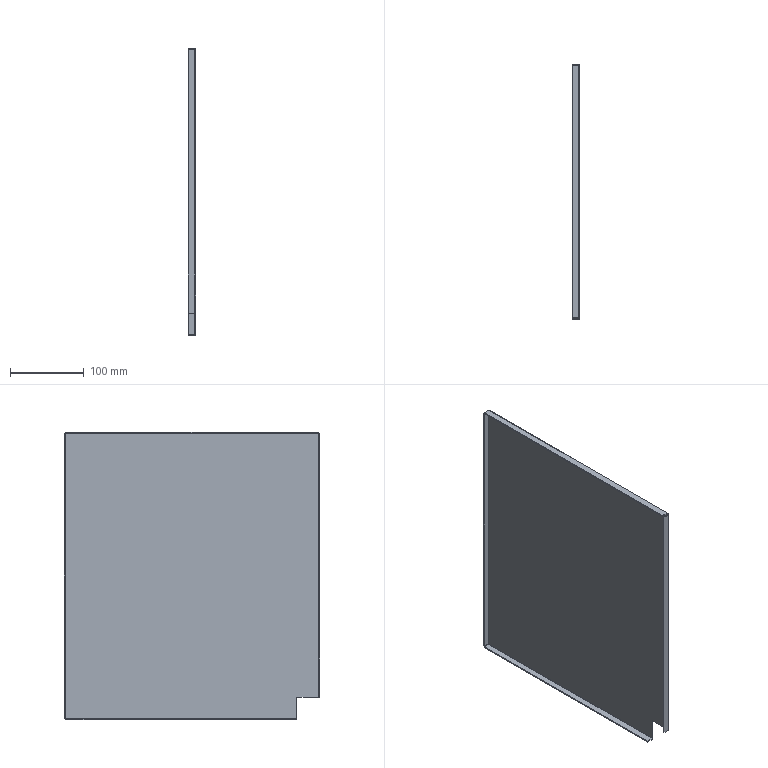Part | SolidWorks | 1 solid | 36 faces | box 10 x 346.001 x 390.001 mm | volume 217996 mm3 | plane 22 | cylinder 8 | spline 6 | commonest cylinder face diameters 0.2 x4 3.2 x4
STEP:
#1=CARTESIAN_POINT('',(-1.5,-142.,-193.4));
#2=VERTEX_POINT('',#1);
#3=CARTESIAN_POINT('',(-1.5,-142.,-164.));
#4=VERTEX_POINT('',#3);
#5=CARTESIAN_POINT('',(-1.5,-142.,0.));
#6=DIRECTION('',(0.,0.,1.));
#7=VECTOR('',#6,1000.);
#8=LINE('',#5,#7);
#9=EDGE_CURVE('',#2,#4,#8,.T.);
#10=ORIENTED_EDGE('',*,*,#9,.T.);
#11=CARTESIAN_POINT('',(-1.5,-171.4,-164.));
#12=VERTEX_POINT('',#11);
#13=CARTESIAN_POINT('',(-1.5,0.,-164.));
#14=DIRECTION('',(0.,-1.,0.));
#15=VECTOR('',#14,1000.);
#16=LINE('',#13,#15);
#17=EDGE_CURVE('',#4,#12,#16,.T.);
#18=ORIENTED_EDGE('',*,*,#17,.T.);
#19=CARTESIAN_POINT('',(-1.5,-171.4,193.4));
#20=VERTEX_POINT('',#19);
#21=CARTESIAN_POINT('',(-1.5,-171.4,193.4));
#22=DIRECTION('',(0.,0.,-1.));
#23=VECTOR('',#22,1000.);
#24=LINE('',#21,#23);
#25=EDGE_CURVE('',#20,#12,#24,.T.);
#26=ORIENTED_EDGE('',*,*,#25,.F.);
#27=CARTESIAN_POINT('',(-1.5,171.4,193.4));
#28=VERTEX_POINT('',#27);
#29=CARTESIAN_POINT('',(-1.5,171.4,193.4));
#30=DIRECTION('',(0.,-1.,0.));
#31=VECTOR('',#30,1000.);
#32=LINE('',#29,#31);
#33=EDGE_CURVE('',#28,#20,#32,.T.);
#34=ORIENTED_EDGE('',*,*,#33,.F.);
#35=CARTESIAN_POINT('',(-1.5,171.4,-193.4));
#36=VERTEX_POINT('',#35);
#37=CARTESIAN_POINT('',(-1.5,171.4,-193.4));
#38=DIRECTION('',(0.,0.,1.));
#39=VECTOR('',#38,1000.);
#40=LINE('',#37,#39);
#41=EDGE_CURVE('',#36,#28,#40,.T.);
#42=ORIENTED_EDGE('',*,*,#41,.F.);
#43=CARTESIAN_POINT('',(-1.5,-171.4,-193.4));
#44=DIRECTION('',(0.,1.,0.));
#45=VECTOR('',#44,1000.);
#46=LINE('',#43,#45);
#47=EDGE_CURVE('',#2,#36,#46,.T.);
#48=ORIENTED_EDGE('',*,*,#47,.F.);
#49=EDGE_LOOP('',(#10,#18,#26,#34,#42,#48));
#50=FACE_OUTER_BOUND('',#49,.T.);
#51=CARTESIAN_POINT('',(-1.5,0.,0.));
#52=DIRECTION('',(1.,0.,0.));
#53=DIRECTION('',(0.,0.,-1.));
#54=AXIS2_PLACEMENT_3D('',#51,#52,#53);
#55=PLANE('',#54);
#56=ADVANCED_FACE('',(#50),#55,.F.);
#57=CARTESIAN_POINT('',(0.,-142.,-164.));
#58=VERTEX_POINT('',#57);
#59=CARTESIAN_POINT('',(0.,-171.4,-164.));
#60=VERTEX_POINT('',#59);
#61=CARTESIAN_POINT('',(0.,-182.,-164.));
#62=DIRECTION('',(0.,-1.,0.));
#63=VECTOR('',#62,1000.);
#64=LINE('',#61,#63);
#65=EDGE_CURVE('',#58,#60,#64,.T.);
#66=ORIENTED_EDGE('',*,*,#65,.F.);
#67=CARTESIAN_POINT('',(0.,-142.,-193.4));
#68=VERTEX_POINT('',#67);
#69=CARTESIAN_POINT('',(0.,-142.,-204.));
#70=DIRECTION('',(0.,0.,1.));
#71=VECTOR('',#70,1000.);
#72=LINE('',#69,#71);
#73=EDGE_CURVE('',#68,#58,#72,.T.);
#74=ORIENTED_EDGE('',*,*,#73,.F.);
#75=CARTESIAN_POINT('',(0.,171.4,-193.4));
#76=VERTEX_POINT('',#75);
#77=CARTESIAN_POINT('',(0.,-171.4,-193.4));
#78=DIRECTION('',(0.,1.,0.));
#79=VECTOR('',#78,1000.);
#80=LINE('',#77,#79);
#81=EDGE_CURVE('',#68,#76,#80,.T.);
#82=ORIENTED_EDGE('',*,*,#81,.T.);
#83=CARTESIAN_POINT('',(0.,171.4,193.4));
#84=VERTEX_POINT('',#83);
#85=CARTESIAN_POINT('',(0.,171.4,-193.4));
#86=DIRECTION('',(0.,0.,1.));
#87=VECTOR('',#86,1000.);
#88=LINE('',#85,#87);
#89=EDGE_CURVE('',#76,#84,#88,.T.);
#90=ORIENTED_EDGE('',*,*,#89,.T.);
#91=CARTESIAN_POINT('',(0.,-171.4,193.4));
#92=VERTEX_POINT('',#91);
#93=CARTESIAN_POINT('',(0.,171.4,193.4));
#94=DIRECTION('',(0.,-1.,0.));
#95=VECTOR('',#94,1000.);
#96=LINE('',#93,#95);
#97=EDGE_CURVE('',#84,#92,#96,.T.);
#98=ORIENTED_EDGE('',*,*,#97,.T.);
#99=CARTESIAN_POINT('',(0.,-171.4,193.4));
#100=DIRECTION('',(0.,0.,-1.));
#101=VECTOR('',#100,1000.);
#102=LINE('',#99,#101);
#103=EDGE_CURVE('',#92,#60,#102,.T.);
#104=ORIENTED_EDGE('',*,*,#103,.T.);
#105=EDGE_LOOP('',(#66,#74,#82,#90,#98,#104));
#106=FACE_OUTER_BOUND('',#105,.T.);
#107=CARTESIAN_POINT('',(0.,0.,0.));
#108=DIRECTION('',(1.,0.,0.));
#109=DIRECTION('',(0.,0.,-1.));
#110=AXIS2_PLACEMENT_3D('',#107,#108,#109);
#111=PLANE('',#110);
#112=ADVANCED_FACE('',(#106),#111,.T.);
#113=CARTESIAN_POINT('',(-1.6,173.,192.793));
#114=VERTEX_POINT('',#113);
#115=CARTESIAN_POINT('',(-1.6,171.5,192.793));
#116=VERTEX_POINT('',#115);
#117=CARTESIAN_POINT('',(-1.6,171.5,192.793));
#118=DIRECTION('',(0.,-1.,0.));
#119=VECTOR('',#118,1000.);
#120=LINE('',#117,#119);
#121=EDGE_CURVE('',#114,#116,#120,.T.);
#122=ORIENTED_EDGE('',*,*,#121,.T.);
#123=CARTESIAN_POINT('',(-1.5,171.4,193.4));
#124=CARTESIAN_POINT('',(-1.5,171.426,193.299));
#125=CARTESIAN_POINT('',(-1.511,171.452,193.198));
#126=CARTESIAN_POINT('',(-1.548,171.489,192.995));
#127=CARTESIAN_POINT('',(-1.574,171.5,192.894));
#128=CARTESIAN_POINT('',(-1.6,171.5,192.793));
#129=B_SPLINE_CURVE_WITH_KNOTS('',3,(#123,#124,#125,#126,#127,#128),.UNSPECIFIED.,.F.,.F.,(4,2,4),(0.,0.5,1.),.UNSPECIFIED.);
#130=EDGE_CURVE('',#28,#116,#129,.T.);
#131=ORIENTED_EDGE('',*,*,#130,.F.);
#132=CARTESIAN_POINT('',(-1.5,171.4,193.4));
#133=DIRECTION('',(1.,0.,0.));
#134=VECTOR('',#133,1000.);
#135=LINE('',#132,#134);
#136=EDGE_CURVE('',#28,#84,#135,.T.);
#137=ORIENTED_EDGE('',*,*,#136,.T.);
#138=CARTESIAN_POINT('',(0.,171.4,193.4));
#139=CARTESIAN_POINT('',(0.,171.612,193.349));
#140=CARTESIAN_POINT('',(-0.04048,171.815,193.3));
#141=CARTESIAN_POINT('',(-0.2012,172.205,193.198));
#142=CARTESIAN_POINT('',(-0.3186,172.381,193.148));
#143=CARTESIAN_POINT('',(-0.5418,172.605,193.071));
#144=CARTESIAN_POINT('',(-0.6225,172.671,193.046));
#145=CARTESIAN_POINT('',(-0.7959,172.787,192.996));
#146=CARTESIAN_POINT('',(-0.8897,172.838,192.97));
#147=CARTESIAN_POINT('',(-1.18,172.958,192.894));
#148=CARTESIAN_POINT('',(-1.388,173.,192.844));
#149=CARTESIAN_POINT('',(-1.6,173.,192.793));
#150=B_SPLINE_CURVE_WITH_KNOTS('',3,(#138,#139,#140,#141,#142,#143,#144,#145,#146,#147,#148,#149),.UNSPECIFIED.,.F.,.F.,(4,2,2,2,2,4),(0.,0.0006399,0.00128,0.0016,0.00192,0.00256),.UNSPECIFIED.);
#151=EDGE_CURVE('',#84,#114,#150,.T.);
#152=ORIENTED_EDGE('',*,*,#151,.T.);
#153=EDGE_LOOP('',(#122,#131,#137,#152));
#154=FACE_OUTER_BOUND('',#153,.T.);
#155=CARTESIAN_POINT('',(0.015,171.4,193.4));
#156=CARTESIAN_POINT('',(0.015,171.611,193.349));
#157=CARTESIAN_POINT('',(-0.02703,171.823,193.299));
#158=CARTESIAN_POINT('',(-0.1888,172.213,193.198));
#159=CARTESIAN_POINT('',(-0.3085,172.392,193.147));
#160=CARTESIAN_POINT('',(-0.6075,172.691,193.046));
#161=CARTESIAN_POINT('',(-0.7867,172.811,192.995));
#162=CARTESIAN_POINT('',(-1.177,172.973,192.894));
#163=CARTESIAN_POINT('',(-1.389,173.015,192.843));
#164=CARTESIAN_POINT('',(-1.6,173.015,192.793));
#165=CARTESIAN_POINT('',(0.,171.4,193.4));
#166=CARTESIAN_POINT('',(0.,171.609,193.349));
#167=CARTESIAN_POINT('',(-0.04164,171.819,193.299));
#168=CARTESIAN_POINT('',(-0.2019,172.206,193.198));
#169=CARTESIAN_POINT('',(-0.3205,172.383,193.147));
#170=CARTESIAN_POINT('',(-0.6167,172.679,193.046));
#171=CARTESIAN_POINT('',(-0.7942,172.798,192.995));
#172=CARTESIAN_POINT('',(-1.181,172.958,192.894));
#173=CARTESIAN_POINT('',(-1.391,173.,192.843));
#174=CARTESIAN_POINT('',(-1.6,173.,192.793));
#175=CARTESIAN_POINT('',(-1.5,171.4,193.4));
#176=CARTESIAN_POINT('',(-1.5,171.413,193.349));
#177=CARTESIAN_POINT('',(-1.503,171.426,193.299));
#178=CARTESIAN_POINT('',(-1.513,171.45,193.198));
#179=CARTESIAN_POINT('',(-1.52,171.461,193.147));
#180=CARTESIAN_POINT('',(-1.539,171.48,193.046));
#181=CARTESIAN_POINT('',(-1.55,171.487,192.995));
#182=CARTESIAN_POINT('',(-1.574,171.497,192.894));
#183=CARTESIAN_POINT('',(-1.587,171.5,192.843));
#184=CARTESIAN_POINT('',(-1.6,171.5,192.793));
#185=B_SPLINE_SURFACE_WITH_KNOTS('',1,3,((#155,#156,#157,#158,#159,#160,#161,#162,#163,#164),(#165,#166,#167,#168,#169,#170,#171,#172,#173,#174),(#175,#176,#177,#178,#179,#180,#181,#182,#183,#184)),.UNSPECIFIED.,.F.,.F.,.F.,(2,1,2),(4,2,2,2,4),(-0.01,0.,1.),(0.,0.25,0.5,0.75,1.),.UNSPECIFIED.);
#186=ADVANCED_FACE('',(#154),#185,.F.);
#187=CARTESIAN_POINT('',(-1.6,171.5,-192.793));
#188=VERTEX_POINT('',#187);
#189=CARTESIAN_POINT('',(-1.6,171.5,-192.793));
#190=CARTESIAN_POINT('',(-1.574,171.5,-192.894));
#191=CARTESIAN_POINT('',(-1.548,171.489,-192.995));
#192=CARTESIAN_POINT('',(-1.511,171.452,-193.198));
#193=CARTESIAN_POINT('',(-1.5,171.426,-193.299));
#194=CARTESIAN_POINT('',(-1.5,171.4,-193.4));
#195=B_SPLINE_CURVE_WITH_KNOTS('',3,(#189,#190,#191,#192,#193,#194),.UNSPECIFIED.,.F.,.F.,(4,2,4),(0.,0.5,1.),.UNSPECIFIED.);
#196=EDGE_CURVE('',#188,#36,#195,.T.);
#197=ORIENTED_EDGE('',*,*,#196,.F.);
#198=CARTESIAN_POINT('',(-1.6,173.,-192.793));
#199=VERTEX_POINT('',#198);
#200=CARTESIAN_POINT('',(-1.6,171.5,-192.793));
#201=DIRECTION('',(0.,-1.,0.));
#202=VECTOR('',#201,1000.);
#203=LINE('',#200,#202);
#204=EDGE_CURVE('',#199,#188,#203,.T.);
#205=ORIENTED_EDGE('',*,*,#204,.F.);
#206=CARTESIAN_POINT('',(-1.6,173.,-192.793));
#207=CARTESIAN_POINT('',(-1.388,173.,-192.844));
#208=CARTESIAN_POINT('',(-1.185,172.96,-192.893));
#209=CARTESIAN_POINT('',(-0.7952,172.799,-192.995));
#210=CARTESIAN_POINT('',(-0.619,172.681,-193.045));
#211=CARTESIAN_POINT('',(-0.3953,172.458,-193.121));
#212=CARTESIAN_POINT('',(-0.329,172.378,-193.147));
#213=CARTESIAN_POINT('',(-0.2128,172.204,-193.197));
#214=CARTESIAN_POINT('',(-0.1625,172.11,-193.223));
#215=CARTESIAN_POINT('',(-0.04195,171.82,-193.299));
#216=CARTESIAN_POINT('',(0.,171.612,-193.349));
#217=CARTESIAN_POINT('',(0.,171.4,-193.4));
#218=B_SPLINE_CURVE_WITH_KNOTS('',3,(#206,#207,#208,#209,#210,#211,#212,#213,#214,#215,#216,#217),.UNSPECIFIED.,.F.,.F.,(4,2,2,2,2,4),(0.,0.0006399,0.00128,0.0016,0.00192,0.00256),.UNSPECIFIED.);
#219=EDGE_CURVE('',#199,#76,#218,.T.);
#220=ORIENTED_EDGE('',*,*,#219,.T.);
#221=CARTESIAN_POINT('',(-1.5,171.4,-193.4));
#222=DIRECTION('',(1.,0.,0.));
#223=VECTOR('',#222,1000.);
#224=LINE('',#221,#223);
#225=EDGE_CURVE('',#36,#76,#224,.T.);
#226=ORIENTED_EDGE('',*,*,#225,.F.);
#227=EDGE_LOOP('',(#197,#205,#220,#226));
#228=FACE_OUTER_BOUND('',#227,.T.);
#229=CARTESIAN_POINT('',(-1.6,173.015,-192.793));
#230=CARTESIAN_POINT('',(-1.389,173.015,-192.843));
#231=CARTESIAN_POINT('',(-1.177,172.973,-192.894));
#232=CARTESIAN_POINT('',(-0.7867,172.811,-192.995));
#233=CARTESIAN_POINT('',(-0.6075,172.691,-193.046));
#234=CARTESIAN_POINT('',(-0.3085,172.392,-193.147));
#235=CARTESIAN_POINT('',(-0.1888,172.213,-193.198));
#236=CARTESIAN_POINT('',(-0.02703,171.823,-193.299));
#237=CARTESIAN_POINT('',(0.015,171.611,-193.349));
#238=CARTESIAN_POINT('',(0.015,171.4,-193.4));
#239=CARTESIAN_POINT('',(-1.6,173.,-192.793));
#240=CARTESIAN_POINT('',(-1.391,173.,-192.843));
#241=CARTESIAN_POINT('',(-1.181,172.958,-192.894));
#242=CARTESIAN_POINT('',(-0.7942,172.798,-192.995));
#243=CARTESIAN_POINT('',(-0.6167,172.679,-193.046));
#244=CARTESIAN_POINT('',(-0.3205,172.383,-193.147));
#245=CARTESIAN_POINT('',(-0.2019,172.206,-193.198));
#246=CARTESIAN_POINT('',(-0.04164,171.819,-193.299));
#247=CARTESIAN_POINT('',(0.,171.609,-193.349));
#248=CARTESIAN_POINT('',(0.,171.4,-193.4));
#249=CARTESIAN_POINT('',(-1.6,171.5,-192.793));
#250=CARTESIAN_POINT('',(-1.587,171.5,-192.843));
#251=CARTESIAN_POINT('',(-1.574,171.497,-192.894));
#252=CARTESIAN_POINT('',(-1.55,171.487,-192.995));
#253=CARTESIAN_POINT('',(-1.539,171.48,-193.046));
#254=CARTESIAN_POINT('',(-1.52,171.461,-193.147));
#255=CARTESIAN_POINT('',(-1.513,171.45,-193.198));
#256=CARTESIAN_POINT('',(-1.503,171.426,-193.299));
#257=CARTESIAN_POINT('',(-1.5,171.413,-193.349));
#258=CARTESIAN_POINT('',(-1.5,171.4,-193.4));
#259=B_SPLINE_SURFACE_WITH_KNOTS('',1,3,((#229,#230,#231,#232,#233,#234,#235,#236,#237,#238),(#239,#240,#241,#242,#243,#244,#245,#246,#247,#248),(#249,#250,#251,#252,#253,#254,#255,#256,#257,#258)),.UNSPECIFIED.,.F.,.F.,.F.,(2,1,2),(4,2,2,2,4),(-0.01,0.,1.),(0.,0.25,0.5,0.75,1.),.UNSPECIFIED.);
#260=ADVANCED_FACE('',(#228),#259,.F.);
#261=ORIENTED_EDGE('',*,*,#89,.F.);
#262=ORIENTED_EDGE('',*,*,#219,.F.);
#263=CARTESIAN_POINT('',(-1.6,173.,0.));
#264=DIRECTION('',(0.,0.,-1.));
#265=VECTOR('',#264,1000.);
#266=LINE('',#263,#265);
#267=EDGE_CURVE('',#114,#199,#266,.T.);
#268=ORIENTED_EDGE('',*,*,#267,.F.);
#269=ORIENTED_EDGE('',*,*,#151,.F.);
#270=EDGE_LOOP('',(#261,#262,#268,#269));
#271=FACE_OUTER_BOUND('',#270,.T.);
#272=CARTESIAN_POINT('',(-1.6,171.4,-193.4));
#273=DIRECTION('',(0.,0.,-1.));
#274=DIRECTION('',(0.,1.,0.));
#275=AXIS2_PLACEMENT_3D('',#272,#273,#274);
#276=CYLINDRICAL_SURFACE('',#275,1.6);
#277=ADVANCED_FACE('',(#271),#276,.T.);
#278=ORIENTED_EDGE('',*,*,#41,.T.);
#279=ORIENTED_EDGE('',*,*,#130,.T.);
#280=CARTESIAN_POINT('',(-1.6,171.5,195.));
#281=DIRECTION('',(0.,0.,-1.));
#282=VECTOR('',#281,1000.);
#283=LINE('',#280,#282);
#284=EDGE_CURVE('',#116,#188,#283,.T.);
#285=ORIENTED_EDGE('',*,*,#284,.T.);
#286=ORIENTED_EDGE('',*,*,#196,.T.);
#287=EDGE_LOOP('',(#278,#279,#285,#286));
#288=FACE_OUTER_BOUND('',#287,.T.);
#289=CARTESIAN_POINT('',(-1.6,171.4,-193.4));
#290=DIRECTION('',(0.,0.,-1.));
#291=DIRECTION('',(0.,1.,0.));
#292=AXIS2_PLACEMENT_3D('',#289,#290,#291);
#293=CYLINDRICAL_SURFACE('',#292,0.1);
#294=ADVANCED_FACE('',(#288),#293,.F.);
#295=CARTESIAN_POINT('',(-10.,171.5,192.793));
#296=VERTEX_POINT('',#295);
#297=CARTESIAN_POINT('',(-10.,173.,192.793));
#298=VERTEX_POINT('',#297);
#299=CARTESIAN_POINT('',(-10.,173.,192.793));
#300=DIRECTION('',(0.,1.,0.));
#301=VECTOR('',#300,1000.);
#302=LINE('',#299,#301);
#303=EDGE_CURVE('',#296,#298,#302,.T.);
#304=ORIENTED_EDGE('',*,*,#303,.F.);
#305=CARTESIAN_POINT('',(0.,171.5,192.793));
#306=DIRECTION('',(-1.,0.,0.));
#307=VECTOR('',#306,1000.);
#308=LINE('',#305,#307);
#309=EDGE_CURVE('',#116,#296,#308,.T.);
#310=ORIENTED_EDGE('',*,*,#309,.F.);
#311=ORIENTED_EDGE('',*,*,#121,.F.);
#312=CARTESIAN_POINT('',(0.,173.,192.793));
#313=DIRECTION('',(1.,0.,0.));
#314=VECTOR('',#313,1000.);
#315=LINE('',#312,#314);
#316=EDGE_CURVE('',#298,#114,#315,.T.);
#317=ORIENTED_EDGE('',*,*,#316,.F.);
#318=EDGE_LOOP('',(#304,#310,#311,#317));
#319=FACE_OUTER_BOUND('',#318,.T.);
#320=CARTESIAN_POINT('',(-1.5,171.5,192.793));
#321=DIRECTION('',(0.,0.,1.));
#322=DIRECTION('',(1.,0.,0.));
#323=AXIS2_PLACEMENT_3D('',#320,#321,#322);
#324=PLANE('',#323);
#325=ADVANCED_FACE('',(#319),#324,.T.);
#326=CARTESIAN_POINT('',(-10.,173.,-192.793));
#327=VERTEX_POINT('',#326);
#328=CARTESIAN_POINT('',(-1.5,173.,-192.793));
#329=DIRECTION('',(1.,0.,0.));
#330=VECTOR('',#329,1000.);
#331=LINE('',#328,#330);
#332=EDGE_CURVE('',#327,#199,#331,.T.);
#333=ORIENTED_EDGE('',*,*,#332,.F.);
#334=CARTESIAN_POINT('',(-10.,173.,-195.));
#335=DIRECTION('',(0.,0.,-1.));
#336=VECTOR('',#335,1000.);
#337=LINE('',#334,#336);
#338=EDGE_CURVE('',#298,#327,#337,.T.);
#339=ORIENTED_EDGE('',*,*,#338,.F.);
#340=ORIENTED_EDGE('',*,*,#316,.T.);
#341=ORIENTED_EDGE('',*,*,#267,.T.);
#342=EDGE_LOOP('',(#333,#339,#340,#341));
#343=FACE_OUTER_BOUND('',#342,.T.);
#344=CARTESIAN_POINT('',(0.,173.,0.));
#345=DIRECTION('',(0.,1.,0.));
#346=DIRECTION('',(-1.,0.,0.));
#347=AXIS2_PLACEMENT_3D('',#344,#345,#346);
#348=PLANE('',#347);
#349=ADVANCED_FACE('',(#343),#348,.T.);
#350=CARTESIAN_POINT('',(-10.,171.5,-192.793));
#351=VERTEX_POINT('',#350);
#352=CARTESIAN_POINT('',(-10.,171.5,0.));
#353=DIRECTION('',(0.,0.,-1.));
#354=VECTOR('',#353,1000.);
#355=LINE('',#352,#354);
#356=EDGE_CURVE('',#296,#351,#355,.T.);
#357=ORIENTED_EDGE('',*,*,#356,.T.);
#358=CARTESIAN_POINT('',(-1.5,171.5,-192.793));
#359=DIRECTION('',(-1.,0.,0.));
#360=VECTOR('',#359,1000.);
#361=LINE('',#358,#360);
#362=EDGE_CURVE('',#188,#351,#361,.T.);
#363=ORIENTED_EDGE('',*,*,#362,.F.);
#364=ORIENTED_EDGE('',*,*,#284,.F.);
#365=ORIENTED_EDGE('',*,*,#309,.T.);
#366=EDGE_LOOP('',(#357,#363,#364,#365));
#367=FACE_OUTER_BOUND('',#366,.T.);
#368=CARTESIAN_POINT('',(0.,171.5,0.));
#369=DIRECTION('',(0.,1.,0.));
#370=DIRECTION('',(-1.,0.,0.));
#371=AXIS2_PLACEMENT_3D('',#368,#369,#370);
#372=PLANE('',#371);
#373=ADVANCED_FACE('',(#367),#372,.F.);
#374=CARTESIAN_POINT('',(-10.,171.5,-192.793));
#375=DIRECTION('',(0.,1.,0.));
#376=VECTOR('',#375,1000.);
#377=LINE('',#374,#376);
#378=EDGE_CURVE('',#351,#327,#377,.T.);
#379=ORIENTED_EDGE('',*,*,#378,.F.);
#380=ORIENTED_EDGE('',*,*,#356,.F.);
#381=ORIENTED_EDGE('',*,*,#303,.T.);
#382=ORIENTED_EDGE('',*,*,#338,.T.);
#383=EDGE_LOOP('',(#379,#380,#381,#382));
#384=FACE_OUTER_BOUND('',#383,.T.);
#385=CARTESIAN_POINT('',(-10.,173.,-195.));
#386=DIRECTION('',(-1.,0.,0.));
#387=DIRECTION('',(0.,-1.,0.));
#388=AXIS2_PLACEMENT_3D('',#385,#386,#387);
#389=PLANE('',#388);
#390=ADVANCED_FACE('',(#384),#389,.T.);
#391=ORIENTED_EDGE('',*,*,#362,.T.);
#392=ORIENTED_EDGE('',*,*,#378,.T.);
#393=ORIENTED_EDGE('',*,*,#332,.T.);
#394=ORIENTED_EDGE('',*,*,#204,.T.);
#395=EDGE_LOOP('',(#391,#392,#393,#394));
#396=FACE_OUTER_BOUND('',#395,.T.);
#397=CARTESIAN_POINT('',(-1.5,171.5,-192.793));
#398=DIRECTION('',(0.,0.,1.));
#399=DIRECTION('',(1.,0.,0.));
#400=AXIS2_PLACEMENT_3D('',#397,#398,#399);
#401=PLANE('',#400);
#402=ADVANCED_FACE('',(#396),#401,.F.);
#403=CARTESIAN_POINT('',(-1.6,-170.793,195.));
#404=VERTEX_POINT('',#403);
#405=CARTESIAN_POINT('',(-1.6,-170.793,193.5));
#406=VERTEX_POINT('',#405);
#407=CARTESIAN_POINT('',(-1.6,-170.793,193.5));
#408=DIRECTION('',(0.,0.,-1.));
#409=VECTOR('',#408,1000.);
#410=LINE('',#407,#409);
#411=EDGE_CURVE('',#404,#406,#410,.T.);
#412=ORIENTED_EDGE('',*,*,#411,.T.);
#413=CARTESIAN_POINT('',(-1.5,-171.4,193.4));
#414=CARTESIAN_POINT('',(-1.5,-171.299,193.426));
#415=CARTESIAN_POINT('',(-1.511,-171.198,193.452));
#416=CARTESIAN_POINT('',(-1.548,-170.995,193.489));
#417=CARTESIAN_POINT('',(-1.574,-170.894,193.5));
#418=CARTESIAN_POINT('',(-1.6,-170.793,193.5));
#419=B_SPLINE_CURVE_WITH_KNOTS('',3,(#413,#414,#415,#416,#417,#418),.UNSPECIFIED.,.F.,.F.,(4,2,4),(0.,0.5,1.),.UNSPECIFIED.);
#420=EDGE_CURVE('',#20,#406,#419,.T.);
#421=ORIENTED_EDGE('',*,*,#420,.F.);
#422=CARTESIAN_POINT('',(-1.5,-171.4,193.4));
#423=DIRECTION('',(1.,0.,0.));
#424=VECTOR('',#423,1000.);
#425=LINE('',#422,#424);
#426=EDGE_CURVE('',#20,#92,#425,.T.);
#427=ORIENTED_EDGE('',*,*,#426,.T.);
#428=CARTESIAN_POINT('',(0.,-171.4,193.4));
#429=CARTESIAN_POINT('',(0.,-171.349,193.612));
#430=CARTESIAN_POINT('',(-0.04048,-171.3,193.815));
#431=CARTESIAN_POINT('',(-0.2012,-171.198,194.205));
#432=CARTESIAN_POINT('',(-0.3186,-171.148,194.381));
#433=CARTESIAN_POINT('',(-0.5418,-171.071,194.605));
#434=CARTESIAN_POINT('',(-0.6225,-171.046,194.671));
#435=CARTESIAN_POINT('',(-0.7959,-170.996,194.787));
#436=CARTESIAN_POINT('',(-0.8897,-170.97,194.838));
#437=CARTESIAN_POINT('',(-1.18,-170.894,194.958));
#438=CARTESIAN_POINT('',(-1.388,-170.844,195.));
#439=CARTESIAN_POINT('',(-1.6,-170.793,195.));
#440=B_SPLINE_CURVE_WITH_KNOTS('',3,(#428,#429,#430,#431,#432,#433,#434,#435,#436,#437,#438,#439),.UNSPECIFIED.,.F.,.F.,(4,2,2,2,2,4),(0.,0.0006399,0.00128,0.0016,0.00192,0.00256),.UNSPECIFIED.);
#441=EDGE_CURVE('',#92,#404,#440,.T.);
#442=ORIENTED_EDGE('',*,*,#441,.T.);
#443=EDGE_LOOP('',(#412,#421,#427,#442));
#444=FACE_OUTER_BOUND('',#443,.T.);
#445=CARTESIAN_POINT('',(0.015,-171.4,193.4));
#446=CARTESIAN_POINT('',(0.015,-171.349,193.611));
#447=CARTESIAN_POINT('',(-0.02703,-171.299,193.823));
#448=CARTESIAN_POINT('',(-0.1888,-171.198,194.213));
#449=CARTESIAN_POINT('',(-0.3085,-171.147,194.392));
#450=CARTESIAN_POINT('',(-0.6075,-171.046,194.691));
#451=CARTESIAN_POINT('',(-0.7867,-170.995,194.811));
#452=CARTESIAN_POINT('',(-1.177,-170.894,194.973));
#453=CARTESIAN_POINT('',(-1.389,-170.843,195.015));
#454=CARTESIAN_POINT('',(-1.6,-170.793,195.015));
#455=CARTESIAN_POINT('',(0.,-171.4,193.4));
#456=CARTESIAN_POINT('',(0.,-171.349,193.609));
#457=CARTESIAN_POINT('',(-0.04164,-171.299,193.819));
#458=CARTESIAN_POINT('',(-0.2019,-171.198,194.206));
#459=CARTESIAN_POINT('',(-0.3205,-171.147,194.383));
#460=CARTESIAN_POINT('',(-0.6167,-171.046,194.679));
#461=CARTESIAN_POINT('',(-0.7942,-170.995,194.798));
#462=CARTESIAN_POINT('',(-1.181,-170.894,194.958));
#463=CARTESIAN_POINT('',(-1.391,-170.843,195.));
#464=CARTESIAN_POINT('',(-1.6,-170.793,195.));
#465=CARTESIAN_POINT('',(-1.5,-171.4,193.4));
#466=CARTESIAN_POINT('',(-1.5,-171.349,193.413));
#467=CARTESIAN_POINT('',(-1.503,-171.299,193.426));
#468=CARTESIAN_POINT('',(-1.513,-171.198,193.45));
#469=CARTESIAN_POINT('',(-1.52,-171.147,193.461));
#470=CARTESIAN_POINT('',(-1.539,-171.046,193.48));
#471=CARTESIAN_POINT('',(-1.55,-170.995,193.487));
#472=CARTESIAN_POINT('',(-1.574,-170.894,193.497));
#473=CARTESIAN_POINT('',(-1.587,-170.843,193.5));
#474=CARTESIAN_POINT('',(-1.6,-170.793,193.5));
#475=B_SPLINE_SURFACE_WITH_KNOTS('',1,3,((#445,#446,#447,#448,#449,#450,#451,#452,#453,#454),(#455,#456,#457,#458,#459,#460,#461,#462,#463,#464),(#465,#466,#467,#468,#469,#470,#471,#472,#473,#474)),.UNSPECIFIED.,.F.,.F.,.F.,(2,1,2),(4,2,2,2,4),(-0.01,0.,1.),(0.,0.25,0.5,0.75,1.),.UNSPECIFIED.);
#476=ADVANCED_FACE('',(#444),#475,.F.);
#477=CARTESIAN_POINT('',(-1.6,170.793,193.5));
#478=VERTEX_POINT('',#477);
#479=CARTESIAN_POINT('',(-1.6,170.793,193.5));
#480=CARTESIAN_POINT('',(-1.574,170.894,193.5));
#481=CARTESIAN_POINT('',(-1.548,170.995,193.489));
#482=CARTESIAN_POINT('',(-1.511,171.198,193.452));
#483=CARTESIAN_POINT('',(-1.5,171.299,193.426));
#484=CARTESIAN_POINT('',(-1.5,171.4,193.4));
#485=B_SPLINE_CURVE_WITH_KNOTS('',3,(#479,#480,#481,#482,#483,#484),.UNSPECIFIED.,.F.,.F.,(4,2,4),(0.,0.5,1.),.UNSPECIFIED.);
#486=EDGE_CURVE('',#478,#28,#485,.T.);
#487=ORIENTED_EDGE('',*,*,#486,.F.);
#488=CARTESIAN_POINT('',(-1.6,170.793,195.));
#489=VERTEX_POINT('',#488);
#490=CARTESIAN_POINT('',(-1.6,170.793,193.5));
#491=DIRECTION('',(0.,0.,-1.));
#492=VECTOR('',#491,1000.);
#493=LINE('',#490,#492);
#494=EDGE_CURVE('',#489,#478,#493,.T.);
#495=ORIENTED_EDGE('',*,*,#494,.F.);
#496=CARTESIAN_POINT('',(-1.6,170.793,195.));
#497=CARTESIAN_POINT('',(-1.388,170.844,195.));
#498=CARTESIAN_POINT('',(-1.185,170.893,194.96));
#499=CARTESIAN_POINT('',(-0.7952,170.995,194.799));
#500=CARTESIAN_POINT('',(-0.619,171.045,194.681));
#501=CARTESIAN_POINT('',(-0.3953,171.121,194.458));
#502=CARTESIAN_POINT('',(-0.329,171.147,194.378));
#503=CARTESIAN_POINT('',(-0.2128,171.197,194.204));
#504=CARTESIAN_POINT('',(-0.1625,171.223,194.11));
#505=CARTESIAN_POINT('',(-0.04195,171.299,193.82));
#506=CARTESIAN_POINT('',(0.,171.349,193.612));
#507=CARTESIAN_POINT('',(0.,171.4,193.4));
#508=B_SPLINE_CURVE_WITH_KNOTS('',3,(#496,#497,#498,#499,#500,#501,#502,#503,#504,#505,#506,#507),.UNSPECIFIED.,.F.,.F.,(4,2,2,2,2,4),(0.,0.0006399,0.00128,0.0016,0.00192,0.00256),.UNSPECIFIED.);
#509=EDGE_CURVE('',#489,#84,#508,.T.);
#510=ORIENTED_EDGE('',*,*,#509,.T.);
#511=ORIENTED_EDGE('',*,*,#136,.F.);
#512=EDGE_LOOP('',(#487,#495,#510,#511));
#513=FACE_OUTER_BOUND('',#512,.T.);
#514=CARTESIAN_POINT('',(-1.6,170.793,195.015));
#515=CARTESIAN_POINT('',(-1.389,170.843,195.015));
#516=CARTESIAN_POINT('',(-1.177,170.894,194.973));
#517=CARTESIAN_POINT('',(-0.7867,170.995,194.811));
#518=CARTESIAN_POINT('',(-0.6075,171.046,194.691));
#519=CARTESIAN_POINT('',(-0.3085,171.147,194.392));
#520=CARTESIAN_POINT('',(-0.1888,171.198,194.213));
#521=CARTESIAN_POINT('',(-0.02703,171.299,193.823));
#522=CARTESIAN_POINT('',(0.015,171.349,193.611));
#523=CARTESIAN_POINT('',(0.015,171.4,193.4));
#524=CARTESIAN_POINT('',(-1.6,170.793,195.));
#525=CARTESIAN_POINT('',(-1.391,170.843,195.));
#526=CARTESIAN_POINT('',(-1.181,170.894,194.958));
#527=CARTESIAN_POINT('',(-0.7942,170.995,194.798));
#528=CARTESIAN_POINT('',(-0.6167,171.046,194.679));
#529=CARTESIAN_POINT('',(-0.3205,171.147,194.383));
#530=CARTESIAN_POINT('',(-0.2019,171.198,194.206));
#531=CARTESIAN_POINT('',(-0.04164,171.299,193.819));
#532=CARTESIAN_POINT('',(0.,171.349,193.609));
#533=CARTESIAN_POINT('',(0.,171.4,193.4));
#534=CARTESIAN_POINT('',(-1.6,170.793,193.5));
#535=CARTESIAN_POINT('',(-1.587,170.843,193.5));
#536=CARTESIAN_POINT('',(-1.574,170.894,193.497));
#537=CARTESIAN_POINT('',(-1.55,170.995,193.487));
#538=CARTESIAN_POINT('',(-1.539,171.046,193.48));
#539=CARTESIAN_POINT('',(-1.52,171.147,193.461));
#540=CARTESIAN_POINT('',(-1.513,171.198,193.45));
#541=CARTESIAN_POINT('',(-1.503,171.299,193.426));
#542=CARTESIAN_POINT('',(-1.5,171.349,193.413));
#543=CARTESIAN_POINT('',(-1.5,171.4,193.4));
#544=B_SPLINE_SURFACE_WITH_KNOTS('',1,3,((#514,#515,#516,#517,#518,#519,#520,#521,#522,#523),(#524,#525,#526,#527,#528,#529,#530,#531,#532,#533),(#534,#535,#536,#537,#538,#539,#540,#541,#542,#543)),.UNSPECIFIED.,.F.,.F.,.F.,(2,1,2),(4,2,2,2,4),(-0.01,0.,1.),(0.,0.25,0.5,0.75,1.),.UNSPECIFIED.);
#545=ADVANCED_FACE('',(#513),#544,.F.);
#546=ORIENTED_EDGE('',*,*,#97,.F.);
#547=ORIENTED_EDGE('',*,*,#509,.F.);
#548=CARTESIAN_POINT('',(-1.6,-173.,195.));
#549=DIRECTION('',(0.,-1.,0.));
#550=VECTOR('',#549,1000.);
#551=LINE('',#548,#550);
#552=EDGE_CURVE('',#489,#404,#551,.T.);
#553=ORIENTED_EDGE('',*,*,#552,.T.);
#554=ORIENTED_EDGE('',*,*,#441,.F.);
#555=EDGE_LOOP('',(#546,#547,#553,#554));
#556=FACE_OUTER_BOUND('',#555,.T.);
#557=CARTESIAN_POINT('',(-1.6,171.4,193.4));
#558=DIRECTION('',(0.,1.,0.));
#559=DIRECTION('',(0.,0.,1.));
#560=AXIS2_PLACEMENT_3D('',#557,#558,#559);
#561=CYLINDRICAL_SURFACE('',#560,1.6);
#562=ADVANCED_FACE('',(#556),#561,.T.);
#563=ORIENTED_EDGE('',*,*,#33,.T.);
#564=ORIENTED_EDGE('',*,*,#420,.T.);
#565=CARTESIAN_POINT('',(-1.6,-173.,193.5));
#566=DIRECTION('',(0.,1.,0.));
#567=VECTOR('',#566,1000.);
#568=LINE('',#565,#567);
#569=EDGE_CURVE('',#406,#478,#568,.T.);
#570=ORIENTED_EDGE('',*,*,#569,.T.);
#571=ORIENTED_EDGE('',*,*,#486,.T.);
#572=EDGE_LOOP('',(#563,#564,#570,#571));
#573=FACE_OUTER_BOUND('',#572,.T.);
#574=CARTESIAN_POINT('',(-1.6,171.4,193.4));
#575=DIRECTION('',(0.,1.,0.));
#576=DIRECTION('',(0.,0.,1.));
#577=AXIS2_PLACEMENT_3D('',#574,#575,#576);
#578=CYLINDRICAL_SURFACE('',#577,0.1);
#579=ADVANCED_FACE('',(#573),#578,.F.);
#580=CARTESIAN_POINT('',(-10.,-170.793,193.5));
#581=VERTEX_POINT('',#580);
#582=CARTESIAN_POINT('',(-10.,-170.793,195.));
#583=VERTEX_POINT('',#582);
#584=CARTESIAN_POINT('',(-10.,-170.793,195.));
#585=DIRECTION('',(0.,0.,1.));
#586=VECTOR('',#585,1000.);
#587=LINE('',#584,#586);
#588=EDGE_CURVE('',#581,#583,#587,.T.);
#589=ORIENTED_EDGE('',*,*,#588,.F.);
#590=CARTESIAN_POINT('',(0.,-170.793,193.5));
#591=DIRECTION('',(-1.,0.,0.));
#592=VECTOR('',#591,1000.);
#593=LINE('',#590,#592);
#594=EDGE_CURVE('',#406,#581,#593,.T.);
#595=ORIENTED_EDGE('',*,*,#594,.F.);
#596=ORIENTED_EDGE('',*,*,#411,.F.);
#597=CARTESIAN_POINT('',(-1.5,-170.793,195.));
#598=DIRECTION('',(-1.,0.,0.));
#599=VECTOR('',#598,1000.);
#600=LINE('',#597,#599);
#601=EDGE_CURVE('',#404,#583,#600,.T.);
#602=ORIENTED_EDGE('',*,*,#601,.T.);
#603=EDGE_LOOP('',(#589,#595,#596,#602));
#604=FACE_OUTER_BOUND('',#603,.T.);
#605=CARTESIAN_POINT('',(-1.5,-170.793,193.5));
#606=DIRECTION('',(0.,-1.,0.));
#607=DIRECTION('',(0.,0.,-1.));
#608=AXIS2_PLACEMENT_3D('',#605,#606,#607);
#609=PLANE('',#608);
#610=ADVANCED_FACE('',(#604),#609,.T.);
#611=ORIENTED_EDGE('',*,*,#552,.F.);
#612=CARTESIAN_POINT('',(-10.,170.793,195.));
#613=VERTEX_POINT('',#612);
#614=CARTESIAN_POINT('',(0.,170.793,195.));
#615=DIRECTION('',(-1.,0.,0.));
#616=VECTOR('',#615,1000.);
#617=LINE('',#614,#616);
#618=EDGE_CURVE('',#489,#613,#617,.T.);
#619=ORIENTED_EDGE('',*,*,#618,.T.);
#620=CARTESIAN_POINT('',(-10.,-173.,195.));
#621=DIRECTION('',(0.,1.,0.));
#622=VECTOR('',#621,1000.);
#623=LINE('',#620,#622);
#624=EDGE_CURVE('',#583,#613,#623,.T.);
#625=ORIENTED_EDGE('',*,*,#624,.F.);
#626=ORIENTED_EDGE('',*,*,#601,.F.);
#627=EDGE_LOOP('',(#611,#619,#625,#626));
#628=FACE_OUTER_BOUND('',#627,.T.);
#629=CARTESIAN_POINT('',(0.,0.,195.));
#630=DIRECTION('',(0.,0.,-1.));
#631=DIRECTION('',(-1.,0.,0.));
#632=AXIS2_PLACEMENT_3D('',#629,#630,#631);
#633=PLANE('',#632);
#634=ADVANCED_FACE('',(#628),#633,.F.);
#635=CARTESIAN_POINT('',(-10.,170.793,193.5));
#636=VERTEX_POINT('',#635);
#637=CARTESIAN_POINT('',(-1.5,170.793,193.5));
#638=DIRECTION('',(-1.,0.,0.));
#639=VECTOR('',#638,1000.);
#640=LINE('',#637,#639);
#641=EDGE_CURVE('',#478,#636,#640,.T.);
#642=ORIENTED_EDGE('',*,*,#641,.F.);
#643=ORIENTED_EDGE('',*,*,#569,.F.);
#644=ORIENTED_EDGE('',*,*,#594,.T.);
#645=CARTESIAN_POINT('',(-10.,0.,193.5));
#646=DIRECTION('',(0.,1.,0.));
#647=VECTOR('',#646,1000.);
#648=LINE('',#645,#647);
#649=EDGE_CURVE('',#581,#636,#648,.T.);
#650=ORIENTED_EDGE('',*,*,#649,.T.);
#651=EDGE_LOOP('',(#642,#643,#644,#650));
#652=FACE_OUTER_BOUND('',#651,.T.);
#653=CARTESIAN_POINT('',(0.,0.,193.5));
#654=DIRECTION('',(0.,0.,-1.));
#655=DIRECTION('',(-1.,0.,0.));
#656=AXIS2_PLACEMENT_3D('',#653,#654,#655);
#657=PLANE('',#656);
#658=ADVANCED_FACE('',(#652),#657,.T.);
#659=CARTESIAN_POINT('',(-10.,170.793,193.5));
#660=DIRECTION('',(0.,0.,1.));
#661=VECTOR('',#660,1000.);
#662=LINE('',#659,#661);
#663=EDGE_CURVE('',#636,#613,#662,.T.);
#664=ORIENTED_EDGE('',*,*,#663,.F.);
#665=ORIENTED_EDGE('',*,*,#649,.F.);
#666=ORIENTED_EDGE('',*,*,#588,.T.);
#667=ORIENTED_EDGE('',*,*,#624,.T.);
#668=EDGE_LOOP('',(#664,#665,#666,#667));
#669=FACE_OUTER_BOUND('',#668,.T.);
#670=CARTESIAN_POINT('',(-10.,-173.,195.));
#671=DIRECTION('',(-1.,0.,0.));
#672=DIRECTION('',(0.,0.,1.));
#673=AXIS2_PLACEMENT_3D('',#670,#671,#672);
#674=PLANE('',#673);
#675=ADVANCED_FACE('',(#669),#674,.T.);
#676=ORIENTED_EDGE('',*,*,#641,.T.);
#677=ORIENTED_EDGE('',*,*,#663,.T.);
#678=ORIENTED_EDGE('',*,*,#618,.F.);
#679=ORIENTED_EDGE('',*,*,#494,.T.);
#680=EDGE_LOOP('',(#676,#677,#678,#679));
#681=FACE_OUTER_BOUND('',#680,.T.);
#682=CARTESIAN_POINT('',(-1.5,170.793,193.5));
#683=DIRECTION('',(0.,-1.,0.));
#684=DIRECTION('',(0.,0.,-1.));
#685=AXIS2_PLACEMENT_3D('',#682,#683,#684);
#686=PLANE('',#685);
#687=ADVANCED_FACE('',(#681),#686,.F.);
#688=CARTESIAN_POINT('',(-1.6,-171.5,192.793));
#689=VERTEX_POINT('',#688);
#690=CARTESIAN_POINT('',(-1.6,-171.5,192.793));
#691=CARTESIAN_POINT('',(-1.574,-171.5,192.894));
#692=CARTESIAN_POINT('',(-1.548,-171.489,192.995));
#693=CARTESIAN_POINT('',(-1.511,-171.452,193.198));
#694=CARTESIAN_POINT('',(-1.5,-171.426,193.299));
#695=CARTESIAN_POINT('',(-1.5,-171.4,193.4));
#696=B_SPLINE_CURVE_WITH_KNOTS('',3,(#690,#691,#692,#693,#694,#695),.UNSPECIFIED.,.F.,.F.,(4,2,4),(0.,0.5,1.),.UNSPECIFIED.);
#697=EDGE_CURVE('',#689,#20,#696,.T.);
#698=ORIENTED_EDGE('',*,*,#697,.F.);
#699=CARTESIAN_POINT('',(-1.6,-173.,192.793));
#700=VERTEX_POINT('',#699);
#701=CARTESIAN_POINT('',(-1.6,-171.5,192.793));
#702=DIRECTION('',(0.,1.,0.));
#703=VECTOR('',#702,1000.);
#704=LINE('',#701,#703);
#705=EDGE_CURVE('',#700,#689,#704,.T.);
#706=ORIENTED_EDGE('',*,*,#705,.F.);
#707=CARTESIAN_POINT('',(-1.6,-173.,192.793));
#708=CARTESIAN_POINT('',(-1.388,-173.,192.844));
#709=CARTESIAN_POINT('',(-1.185,-172.96,192.893));
#710=CARTESIAN_POINT('',(-0.7952,-172.799,192.995));
#711=CARTESIAN_POINT('',(-0.619,-172.681,193.045));
#712=CARTESIAN_POINT('',(-0.3953,-172.458,193.121));
#713=CARTESIAN_POINT('',(-0.329,-172.378,193.147));
#714=CARTESIAN_POINT('',(-0.2128,-172.204,193.197));
#715=CARTESIAN_POINT('',(-0.1625,-172.11,193.223));
#716=CARTESIAN_POINT('',(-0.04195,-171.82,193.299));
#717=CARTESIAN_POINT('',(0.,-171.612,193.349));
#718=CARTESIAN_POINT('',(0.,-171.4,193.4));
#719=B_SPLINE_CURVE_WITH_KNOTS('',3,(#707,#708,#709,#710,#711,#712,#713,#714,#715,#716,#717,#718),.UNSPECIFIED.,.F.,.F.,(4,2,2,2,2,4),(0.,0.0006399,0.00128,0.0016,0.00192,0.00256),.UNSPECIFIED.);
#720=EDGE_CURVE('',#700,#92,#719,.T.);
#721=ORIENTED_EDGE('',*,*,#720,.T.);
#722=ORIENTED_EDGE('',*,*,#426,.F.);
#723=EDGE_LOOP('',(#698,#706,#721,#722));
#724=FACE_OUTER_BOUND('',#723,.T.);
#725=CARTESIAN_POINT('',(-1.6,-173.015,192.793));
#726=CARTESIAN_POINT('',(-1.389,-173.015,192.843));
#727=CARTESIAN_POINT('',(-1.177,-172.973,192.894));
#728=CARTESIAN_POINT('',(-0.7867,-172.811,192.995));
#729=CARTESIAN_POINT('',(-0.6075,-172.691,193.046));
#730=CARTESIAN_POINT('',(-0.3085,-172.392,193.147));
#731=CARTESIAN_POINT('',(-0.1888,-172.213,193.198));
#732=CARTESIAN_POINT('',(-0.02703,-171.823,193.299));
#733=CARTESIAN_POINT('',(0.015,-171.611,193.349));
#734=CARTESIAN_POINT('',(0.015,-171.4,193.4));
#735=CARTESIAN_POINT('',(-1.6,-173.,192.793));
#736=CARTESIAN_POINT('',(-1.391,-173.,192.843));
#737=CARTESIAN_POINT('',(-1.181,-172.958,192.894));
#738=CARTESIAN_POINT('',(-0.7942,-172.798,192.995));
#739=CARTESIAN_POINT('',(-0.6167,-172.679,193.046));
#740=CARTESIAN_POINT('',(-0.3205,-172.383,193.147));
#741=CARTESIAN_POINT('',(-0.2019,-172.206,193.198));
#742=CARTESIAN_POINT('',(-0.04164,-171.819,193.299));
#743=CARTESIAN_POINT('',(0.,-171.609,193.349));
#744=CARTESIAN_POINT('',(0.,-171.4,193.4));
#745=CARTESIAN_POINT('',(-1.6,-171.5,192.793));
#746=CARTESIAN_POINT('',(-1.587,-171.5,192.843));
#747=CARTESIAN_POINT('',(-1.574,-171.497,192.894));
#748=CARTESIAN_POINT('',(-1.55,-171.487,192.995));
#749=CARTESIAN_POINT('',(-1.539,-171.48,193.046));
#750=CARTESIAN_POINT('',(-1.52,-171.461,193.147));
#751=CARTESIAN_POINT('',(-1.513,-171.45,193.198));
#752=CARTESIAN_POINT('',(-1.503,-171.426,193.299));
#753=CARTESIAN_POINT('',(-1.5,-171.413,193.349));
#754=CARTESIAN_POINT('',(-1.5,-171.4,193.4));
#755=B_SPLINE_SURFACE_WITH_KNOTS('',1,3,((#725,#726,#727,#728,#729,#730,#731,#732,#733,#734),(#735,#736,#737,#738,#739,#740,#741,#742,#743,#744),(#745,#746,#747,#748,#749,#750,#751,#752,#753,#754)),.UNSPECIFIED.,.F.,.F.,.F.,(2,1,2),(4,2,2,2,4),(-0.01,0.,1.),(0.,0.25,0.5,0.75,1.),.UNSPECIFIED.);
#756=ADVANCED_FACE('',(#724),#755,.F.);
#757=CARTESIAN_POINT('',(-1.6,-173.,-164.));
#758=VERTEX_POINT('',#757);
#759=CARTESIAN_POINT('',(-1.6,-171.4,-164.));
#760=DIRECTION('',(0.,0.,-1.));
#761=DIRECTION('',(0.,-1.,0.));
#762=AXIS2_PLACEMENT_3D('',#759,#760,#761);
#763=CIRCLE('',#762,1.6);
#764=EDGE_CURVE('',#60,#758,#763,.T.);
#765=ORIENTED_EDGE('',*,*,#764,.F.);
#766=ORIENTED_EDGE('',*,*,#103,.F.);
#767=ORIENTED_EDGE('',*,*,#720,.F.);
#768=CARTESIAN_POINT('',(-1.6,-173.,-195.));
#769=DIRECTION('',(0.,0.,-1.));
#770=VECTOR('',#769,1000.);
#771=LINE('',#768,#770);
#772=EDGE_CURVE('',#700,#758,#771,.T.);
#773=ORIENTED_EDGE('',*,*,#772,.T.);
#774=EDGE_LOOP('',(#765,#766,#767,#773));
#775=FACE_OUTER_BOUND('',#774,.T.);
#776=CARTESIAN_POINT('',(-1.6,-171.4,193.4));
#777=DIRECTION('',(0.,0.,1.));
#778=DIRECTION('',(0.,-1.,0.));
#779=AXIS2_PLACEMENT_3D('',#776,#777,#778);
#780=CYLINDRICAL_SURFACE('',#779,1.6);
#781=ADVANCED_FACE('',(#775),#780,.T.);
#782=ORIENTED_EDGE('',*,*,#25,.T.);
#783=CARTESIAN_POINT('',(-1.6,-171.5,-164.));
#784=VERTEX_POINT('',#783);
#785=CARTESIAN_POINT('',(-1.6,-171.4,-164.));
#786=DIRECTION('',(0.,0.,-1.));
#787=DIRECTION('',(0.,-1.,0.));
#788=AXIS2_PLACEMENT_3D('',#785,#786,#787);
#789=CIRCLE('',#788,0.1);
#790=EDGE_CURVE('',#12,#784,#789,.T.);
#791=ORIENTED_EDGE('',*,*,#790,.T.);
#792=CARTESIAN_POINT('',(-1.6,-171.5,-195.));
#793=DIRECTION('',(0.,0.,1.));
#794=VECTOR('',#793,1000.);
#795=LINE('',#792,#794);
#796=EDGE_CURVE('',#784,#689,#795,.T.);
#797=ORIENTED_EDGE('',*,*,#796,.T.);
#798=ORIENTED_EDGE('',*,*,#697,.T.);
#799=EDGE_LOOP('',(#782,#791,#797,#798));
#800=FACE_OUTER_BOUND('',#799,.T.);
#801=CARTESIAN_POINT('',(-1.6,-171.4,193.4));
#802=DIRECTION('',(0.,0.,1.));
#803=DIRECTION('',(0.,-1.,0.));
#804=AXIS2_PLACEMENT_3D('',#801,#802,#803);
#805=CYLINDRICAL_SURFACE('',#804,0.1);
#806=ADVANCED_FACE('',(#800),#805,.F.);
#807=CARTESIAN_POINT('',(-10.,-173.,-164.));
#808=VERTEX_POINT('',#807);
#809=CARTESIAN_POINT('',(-10.,-173.,192.793));
#810=VERTEX_POINT('',#809);
#811=CARTESIAN_POINT('',(-10.,-173.,-195.));
#812=DIRECTION('',(0.,0.,1.));
#813=VECTOR('',#812,1000.);
#814=LINE('',#811,#813);
#815=EDGE_CURVE('',#808,#810,#814,.T.);
#816=ORIENTED_EDGE('',*,*,#815,.F.);
#817=CARTESIAN_POINT('',(0.,-173.,-164.));
#818=DIRECTION('',(1.,0.,0.));
#819=VECTOR('',#818,1000.);
#820=LINE('',#817,#819);
#821=EDGE_CURVE('',#808,#758,#820,.T.);
#822=ORIENTED_EDGE('',*,*,#821,.T.);
#823=ORIENTED_EDGE('',*,*,#772,.F.);
#824=CARTESIAN_POINT('',(0.,-173.,192.793));
#825=DIRECTION('',(-1.,0.,0.));
#826=VECTOR('',#825,1000.);
#827=LINE('',#824,#826);
#828=EDGE_CURVE('',#700,#810,#827,.T.);
#829=ORIENTED_EDGE('',*,*,#828,.T.);
#830=EDGE_LOOP('',(#816,#822,#823,#829));
#831=FACE_OUTER_BOUND('',#830,.T.);
#832=CARTESIAN_POINT('',(0.,-173.,0.));
#833=DIRECTION('',(0.,1.,0.));
#834=DIRECTION('',(-1.,0.,0.));
#835=AXIS2_PLACEMENT_3D('',#832,#833,#834);
#836=PLANE('',#835);
#837=ADVANCED_FACE('',(#831),#836,.F.);
#838=CARTESIAN_POINT('',(-10.,-171.5,-164.));
#839=VERTEX_POINT('',#838);
#840=CARTESIAN_POINT('',(0.,-171.5,-164.));
#841=DIRECTION('',(1.,0.,0.));
#842=VECTOR('',#841,1000.);
#843=LINE('',#840,#842);
#844=EDGE_CURVE('',#839,#784,#843,.T.);
#845=ORIENTED_EDGE('',*,*,#844,.F.);
#846=CARTESIAN_POINT('',(-10.,-171.5,192.793));
#847=VERTEX_POINT('',#846);
#848=CARTESIAN_POINT('',(-10.,-171.5,0.));
#849=DIRECTION('',(0.,0.,1.));
#850=VECTOR('',#849,1000.);
#851=LINE('',#848,#850);
#852=EDGE_CURVE('',#839,#847,#851,.T.);
#853=ORIENTED_EDGE('',*,*,#852,.T.);
#854=CARTESIAN_POINT('',(-1.5,-171.5,192.793));
#855=DIRECTION('',(-1.,0.,0.));
#856=VECTOR('',#855,1000.);
#857=LINE('',#854,#856);
#858=EDGE_CURVE('',#689,#847,#857,.T.);
#859=ORIENTED_EDGE('',*,*,#858,.F.);
#860=ORIENTED_EDGE('',*,*,#796,.F.);
#861=EDGE_LOOP('',(#845,#853,#859,#860));
#862=FACE_OUTER_BOUND('',#861,.T.);
#863=CARTESIAN_POINT('',(0.,-171.5,0.));
#864=DIRECTION('',(0.,1.,0.));
#865=DIRECTION('',(-1.,0.,0.));
#866=AXIS2_PLACEMENT_3D('',#863,#864,#865);
#867=PLANE('',#866);
#868=ADVANCED_FACE('',(#862),#867,.T.);
#869=CARTESIAN_POINT('',(-10.,-182.,-164.));
#870=DIRECTION('',(0.,-1.,0.));
#871=VECTOR('',#870,1000.);
#872=LINE('',#869,#871);
#873=EDGE_CURVE('',#839,#808,#872,.T.);
#874=ORIENTED_EDGE('',*,*,#873,.T.);
#875=ORIENTED_EDGE('',*,*,#815,.T.);
#876=CARTESIAN_POINT('',(-10.,-171.5,192.793));
#877=DIRECTION('',(0.,-1.,0.));
#878=VECTOR('',#877,1000.);
#879=LINE('',#876,#878);
#880=EDGE_CURVE('',#847,#810,#879,.T.);
#881=ORIENTED_EDGE('',*,*,#880,.F.);
#882=ORIENTED_EDGE('',*,*,#852,.F.);
#883=EDGE_LOOP('',(#874,#875,#881,#882));
#884=FACE_OUTER_BOUND('',#883,.T.);
#885=CARTESIAN_POINT('',(-10.,-173.,-195.));
#886=DIRECTION('',(-1.,0.,0.));
#887=DIRECTION('',(0.,-1.,0.));
#888=AXIS2_PLACEMENT_3D('',#885,#886,#887);
#889=PLANE('',#888);
#890=ADVANCED_FACE('',(#884),#889,.T.);
#891=ORIENTED_EDGE('',*,*,#858,.T.);
#892=ORIENTED_EDGE('',*,*,#880,.T.);
#893=ORIENTED_EDGE('',*,*,#828,.F.);
#894=ORIENTED_EDGE('',*,*,#705,.T.);
#895=EDGE_LOOP('',(#891,#892,#893,#894));
#896=FACE_OUTER_BOUND('',#895,.T.);
#897=CARTESIAN_POINT('',(-1.5,-171.5,192.793));
#898=DIRECTION('',(0.,0.,-1.));
#899=DIRECTION('',(-1.,0.,0.));
#900=AXIS2_PLACEMENT_3D('',#897,#898,#899);
#901=PLANE('',#900);
#902=ADVANCED_FACE('',(#896),#901,.F.);
#903=CARTESIAN_POINT('',(-1.6,170.793,-195.));
#904=VERTEX_POINT('',#903);
#905=CARTESIAN_POINT('',(-1.6,170.793,-193.5));
#906=VERTEX_POINT('',#905);
#907=CARTESIAN_POINT('',(-1.6,170.793,-193.5));
#908=DIRECTION('',(0.,0.,1.));
#909=VECTOR('',#908,1000.);
#910=LINE('',#907,#909);
#911=EDGE_CURVE('',#904,#906,#910,.T.);
#912=ORIENTED_EDGE('',*,*,#911,.T.);
#913=CARTESIAN_POINT('',(-1.5,171.4,-193.4));
#914=CARTESIAN_POINT('',(-1.5,171.299,-193.426));
#915=CARTESIAN_POINT('',(-1.511,171.198,-193.452));
#916=CARTESIAN_POINT('',(-1.548,170.995,-193.489));
#917=CARTESIAN_POINT('',(-1.574,170.894,-193.5));
#918=CARTESIAN_POINT('',(-1.6,170.793,-193.5));
#919=B_SPLINE_CURVE_WITH_KNOTS('',3,(#913,#914,#915,#916,#917,#918),.UNSPECIFIED.,.F.,.F.,(4,2,4),(0.,0.5,1.),.UNSPECIFIED.);
#920=EDGE_CURVE('',#36,#906,#919,.T.);
#921=ORIENTED_EDGE('',*,*,#920,.F.);
#922=ORIENTED_EDGE('',*,*,#225,.T.);
#923=CARTESIAN_POINT('',(0.,171.4,-193.4));
#924=CARTESIAN_POINT('',(0.,171.349,-193.612));
#925=CARTESIAN_POINT('',(-0.04048,171.3,-193.815));
#926=CARTESIAN_POINT('',(-0.2012,171.198,-194.205));
#927=CARTESIAN_POINT('',(-0.3186,171.148,-194.381));
#928=CARTESIAN_POINT('',(-0.5418,171.071,-194.605));
#929=CARTESIAN_POINT('',(-0.6225,171.046,-194.671));
#930=CARTESIAN_POINT('',(-0.7959,170.996,-194.787));
#931=CARTESIAN_POINT('',(-0.8897,170.97,-194.838));
#932=CARTESIAN_POINT('',(-1.18,170.894,-194.958));
#933=CARTESIAN_POINT('',(-1.388,170.844,-195.));
#934=CARTESIAN_POINT('',(-1.6,170.793,-195.));
#935=B_SPLINE_CURVE_WITH_KNOTS('',3,(#923,#924,#925,#926,#927,#928,#929,#930,#931,#932,#933,#934),.UNSPECIFIED.,.F.,.F.,(4,2,2,2,2,4),(0.,0.0006399,0.00128,0.0016,0.00192,0.00256),.UNSPECIFIED.);
#936=EDGE_CURVE('',#76,#904,#935,.T.);
#937=ORIENTED_EDGE('',*,*,#936,.T.);
#938=EDGE_LOOP('',(#912,#921,#922,#937));
#939=FACE_OUTER_BOUND('',#938,.T.);
#940=CARTESIAN_POINT('',(0.015,171.4,-193.4));
#941=CARTESIAN_POINT('',(0.015,171.349,-193.611));
#942=CARTESIAN_POINT('',(-0.02703,171.299,-193.823));
#943=CARTESIAN_POINT('',(-0.1888,171.198,-194.213));
#944=CARTESIAN_POINT('',(-0.3085,171.147,-194.392));
#945=CARTESIAN_POINT('',(-0.6075,171.046,-194.691));
#946=CARTESIAN_POINT('',(-0.7867,170.995,-194.811));
#947=CARTESIAN_POINT('',(-1.177,170.894,-194.973));
#948=CARTESIAN_POINT('',(-1.389,170.843,-195.015));
#949=CARTESIAN_POINT('',(-1.6,170.793,-195.015));
#950=CARTESIAN_POINT('',(0.,171.4,-193.4));
#951=CARTESIAN_POINT('',(0.,171.349,-193.609));
#952=CARTESIAN_POINT('',(-0.04164,171.299,-193.819));
#953=CARTESIAN_POINT('',(-0.2019,171.198,-194.206));
#954=CARTESIAN_POINT('',(-0.3205,171.147,-194.383));
#955=CARTESIAN_POINT('',(-0.6167,171.046,-194.679));
#956=CARTESIAN_POINT('',(-0.7942,170.995,-194.798));
#957=CARTESIAN_POINT('',(-1.181,170.894,-194.958));
#958=CARTESIAN_POINT('',(-1.391,170.843,-195.));
#959=CARTESIAN_POINT('',(-1.6,170.793,-195.));
#960=CARTESIAN_POINT('',(-1.5,171.4,-193.4));
#961=CARTESIAN_POINT('',(-1.5,171.349,-193.413));
#962=CARTESIAN_POINT('',(-1.503,171.299,-193.426));
#963=CARTESIAN_POINT('',(-1.513,171.198,-193.45));
#964=CARTESIAN_POINT('',(-1.52,171.147,-193.461));
#965=CARTESIAN_POINT('',(-1.539,171.046,-193.48));
#966=CARTESIAN_POINT('',(-1.55,170.995,-193.487));
#967=CARTESIAN_POINT('',(-1.574,170.894,-193.497));
#968=CARTESIAN_POINT('',(-1.587,170.843,-193.5));
#969=CARTESIAN_POINT('',(-1.6,170.793,-193.5));
#970=B_SPLINE_SURFACE_WITH_KNOTS('',1,3,((#940,#941,#942,#943,#944,#945,#946,#947,#948,#949),(#950,#951,#952,#953,#954,#955,#956,#957,#958,#959),(#960,#961,#962,#963,#964,#965,#966,#967,#968,#969)),.UNSPECIFIED.,.F.,.F.,.F.,(2,1,2),(4,2,2,2,4),(-0.01,0.,1.),(0.,0.25,0.5,0.75,1.),.UNSPECIFIED.);
#971=ADVANCED_FACE('',(#939),#970,.F.);
#972=CARTESIAN_POINT('',(-1.6,-142.,-195.));
#973=VERTEX_POINT('',#972);
#974=CARTESIAN_POINT('',(-1.6,-142.,-193.4));
#975=DIRECTION('',(0.,-1.,0.));
#976=DIRECTION('',(0.,0.,1.));
#977=AXIS2_PLACEMENT_3D('',#974,#975,#976);
#978=CIRCLE('',#977,1.6);
#979=EDGE_CURVE('',#973,#68,#978,.T.);
#980=ORIENTED_EDGE('',*,*,#979,.F.);
#981=CARTESIAN_POINT('',(-1.6,173.,-195.));
#982=DIRECTION('',(0.,1.,0.));
#983=VECTOR('',#982,1000.);
#984=LINE('',#981,#983);
#985=EDGE_CURVE('',#973,#904,#984,.T.);
#986=ORIENTED_EDGE('',*,*,#985,.T.);
#987=ORIENTED_EDGE('',*,*,#936,.F.);
#988=ORIENTED_EDGE('',*,*,#81,.F.);
#989=EDGE_LOOP('',(#980,#986,#987,#988));
#990=FACE_OUTER_BOUND('',#989,.T.);
#991=CARTESIAN_POINT('',(-1.6,-171.4,-193.4));
#992=DIRECTION('',(0.,-1.,0.));
#993=DIRECTION('',(0.,0.,-1.));
#994=AXIS2_PLACEMENT_3D('',#991,#992,#993);
#995=CYLINDRICAL_SURFACE('',#994,1.6);
#996=ADVANCED_FACE('',(#990),#995,.T.);
#997=CARTESIAN_POINT('',(-1.6,-142.,-193.5));
#998=VERTEX_POINT('',#997);
#999=CARTESIAN_POINT('',(-1.6,173.,-193.5));
#1000=DIRECTION('',(0.,-1.,0.));
#1001=VECTOR('',#1000,1000.);
#1002=LINE('',#999,#1001);
#1003=EDGE_CURVE('',#906,#998,#1002,.T.);
#1004=ORIENTED_EDGE('',*,*,#1003,.T.);
#1005=CARTESIAN_POINT('',(-1.6,-142.,-193.4));
#1006=DIRECTION('',(0.,-1.,0.));
#1007=DIRECTION('',(0.,0.,1.));
#1008=AXIS2_PLACEMENT_3D('',#1005,#1006,#1007);
#1009=CIRCLE('',#1008,0.1);
#1010=EDGE_CURVE('',#998,#2,#1009,.T.);
#1011=ORIENTED_EDGE('',*,*,#1010,.T.);
#1012=ORIENTED_EDGE('',*,*,#47,.T.);
#1013=ORIENTED_EDGE('',*,*,#920,.T.);
#1014=EDGE_LOOP('',(#1004,#1011,#1012,#1013));
#1015=FACE_OUTER_BOUND('',#1014,.T.);
#1016=CARTESIAN_POINT('',(-1.6,-171.4,-193.4));
#1017=DIRECTION('',(0.,-1.,0.));
#1018=DIRECTION('',(0.,0.,-1.));
#1019=AXIS2_PLACEMENT_3D('',#1016,#1017,#1018);
#1020=CYLINDRICAL_SURFACE('',#1019,0.1);
#1021=ADVANCED_FACE('',(#1015),#1020,.F.);
#1022=CARTESIAN_POINT('',(-10.,170.793,-193.5));
#1023=VERTEX_POINT('',#1022);
#1024=CARTESIAN_POINT('',(-10.,170.793,-195.));
#1025=VERTEX_POINT('',#1024);
#1026=CARTESIAN_POINT('',(-10.,170.793,-195.));
#1027=DIRECTION('',(0.,0.,-1.));
#1028=VECTOR('',#1027,1000.);
#1029=LINE('',#1026,#1028);
#1030=EDGE_CURVE('',#1023,#1025,#1029,.T.);
#1031=ORIENTED_EDGE('',*,*,#1030,.F.);
#1032=CARTESIAN_POINT('',(0.,170.793,-193.5));
#1033=DIRECTION('',(-1.,0.,0.));
#1034=VECTOR('',#1033,1000.);
#1035=LINE('',#1032,#1034);
#1036=EDGE_CURVE('',#906,#1023,#1035,.T.);
#1037=ORIENTED_EDGE('',*,*,#1036,.F.);
#1038=ORIENTED_EDGE('',*,*,#911,.F.);
#1039=CARTESIAN_POINT('',(-1.5,170.793,-195.));
#1040=DIRECTION('',(-1.,0.,0.));
#1041=VECTOR('',#1040,1000.);
#1042=LINE('',#1039,#1041);
#1043=EDGE_CURVE('',#904,#1025,#1042,.T.);
#1044=ORIENTED_EDGE('',*,*,#1043,.T.);
#1045=EDGE_LOOP('',(#1031,#1037,#1038,#1044));
#1046=FACE_OUTER_BOUND('',#1045,.T.);
#1047=CARTESIAN_POINT('',(-1.5,170.793,-193.5));
#1048=DIRECTION('',(0.,1.,0.));
#1049=DIRECTION('',(0.,0.,1.));
#1050=AXIS2_PLACEMENT_3D('',#1047,#1048,#1049);
#1051=PLANE('',#1050);
#1052=ADVANCED_FACE('',(#1046),#1051,.T.);
#1053=ORIENTED_EDGE('',*,*,#985,.F.);
#1054=CARTESIAN_POINT('',(-10.,-142.,-195.));
#1055=VERTEX_POINT('',#1054);
#1056=CARTESIAN_POINT('',(0.,-142.,-195.));
#1057=DIRECTION('',(-1.,0.,0.));
#1058=VECTOR('',#1057,1000.);
#1059=LINE('',#1056,#1058);
#1060=EDGE_CURVE('',#973,#1055,#1059,.T.);
#1061=ORIENTED_EDGE('',*,*,#1060,.T.);
#1062=CARTESIAN_POINT('',(-10.,173.,-195.));
#1063=DIRECTION('',(0.,-1.,0.));
#1064=VECTOR('',#1063,1000.);
#1065=LINE('',#1062,#1064);
#1066=EDGE_CURVE('',#1025,#1055,#1065,.T.);
#1067=ORIENTED_EDGE('',*,*,#1066,.F.);
#1068=ORIENTED_EDGE('',*,*,#1043,.F.);
#1069=EDGE_LOOP('',(#1053,#1061,#1067,#1068));
#1070=FACE_OUTER_BOUND('',#1069,.T.);
#1071=CARTESIAN_POINT('',(0.,0.,-195.));
#1072=DIRECTION('',(0.,0.,1.));
#1073=DIRECTION('',(1.,0.,0.));
#1074=AXIS2_PLACEMENT_3D('',#1071,#1072,#1073);
#1075=PLANE('',#1074);
#1076=ADVANCED_FACE('',(#1070),#1075,.F.);
#1077=CARTESIAN_POINT('',(-10.,-142.,-193.5));
#1078=VERTEX_POINT('',#1077);
#1079=CARTESIAN_POINT('',(0.,-142.,-193.5));
#1080=DIRECTION('',(-1.,0.,0.));
#1081=VECTOR('',#1080,1000.);
#1082=LINE('',#1079,#1081);
#1083=EDGE_CURVE('',#998,#1078,#1082,.T.);
#1084=ORIENTED_EDGE('',*,*,#1083,.F.);
#1085=ORIENTED_EDGE('',*,*,#1003,.F.);
#1086=ORIENTED_EDGE('',*,*,#1036,.T.);
#1087=CARTESIAN_POINT('',(-10.,0.,-193.5));
#1088=DIRECTION('',(0.,-1.,0.));
#1089=VECTOR('',#1088,1000.);
#1090=LINE('',#1087,#1089);
#1091=EDGE_CURVE('',#1023,#1078,#1090,.T.);
#1092=ORIENTED_EDGE('',*,*,#1091,.T.);
#1093=EDGE_LOOP('',(#1084,#1085,#1086,#1092));
#1094=FACE_OUTER_BOUND('',#1093,.T.);
#1095=CARTESIAN_POINT('',(0.,0.,-193.5));
#1096=DIRECTION('',(0.,0.,1.));
#1097=DIRECTION('',(1.,0.,0.));
#1098=AXIS2_PLACEMENT_3D('',#1095,#1096,#1097);
#1099=PLANE('',#1098);
#1100=ADVANCED_FACE('',(#1094),#1099,.T.);
#1101=CARTESIAN_POINT('',(-10.,-142.,-204.));
#1102=DIRECTION('',(0.,0.,1.));
#1103=VECTOR('',#1102,1000.);
#1104=LINE('',#1101,#1103);
#1105=EDGE_CURVE('',#1055,#1078,#1104,.T.);
#1106=ORIENTED_EDGE('',*,*,#1105,.T.);
#1107=ORIENTED_EDGE('',*,*,#1091,.F.);
#1108=ORIENTED_EDGE('',*,*,#1030,.T.);
#1109=ORIENTED_EDGE('',*,*,#1066,.T.);
#1110=EDGE_LOOP('',(#1106,#1107,#1108,#1109));
#1111=FACE_OUTER_BOUND('',#1110,.T.);
#1112=CARTESIAN_POINT('',(-10.,173.,-195.));
#1113=DIRECTION('',(-1.,0.,0.));
#1114=DIRECTION('',(0.,0.,1.));
#1115=AXIS2_PLACEMENT_3D('',#1112,#1113,#1114);
#1116=PLANE('',#1115);
#1117=ADVANCED_FACE('',(#1111),#1116,.T.);
#1118=ORIENTED_EDGE('',*,*,#764,.T.);
#1119=ORIENTED_EDGE('',*,*,#821,.F.);
#1120=ORIENTED_EDGE('',*,*,#873,.F.);
#1121=ORIENTED_EDGE('',*,*,#844,.T.);
#1122=ORIENTED_EDGE('',*,*,#790,.F.);
#1123=ORIENTED_EDGE('',*,*,#17,.F.);
#1124=CARTESIAN_POINT('',(-10.,-142.,-164.));
#1125=DIRECTION('',(1.,0.,0.));
#1126=VECTOR('',#1125,1000.);
#1127=LINE('',#1124,#1126);
#1128=EDGE_CURVE('',#4,#58,#1127,.T.);
#1129=ORIENTED_EDGE('',*,*,#1128,.T.);
#1130=ORIENTED_EDGE('',*,*,#65,.T.);
#1131=EDGE_LOOP('',(#1118,#1119,#1120,#1121,#1122,#1123,#1129,#1130));
#1132=FACE_OUTER_BOUND('',#1131,.T.);
#1133=CARTESIAN_POINT('',(-10.,-182.,-164.));
#1134=DIRECTION('',(0.,0.,1.));
#1135=DIRECTION('',(0.,-1.,0.));
#1136=AXIS2_PLACEMENT_3D('',#1133,#1134,#1135);
#1137=PLANE('',#1136);
#1138=ADVANCED_FACE('',(#1132),#1137,.F.);
#1139=ORIENTED_EDGE('',*,*,#979,.T.);
#1140=ORIENTED_EDGE('',*,*,#73,.T.);
#1141=ORIENTED_EDGE('',*,*,#1128,.F.);
#1142=ORIENTED_EDGE('',*,*,#9,.F.);
#1143=ORIENTED_EDGE('',*,*,#1010,.F.);
#1144=ORIENTED_EDGE('',*,*,#1083,.T.);
#1145=ORIENTED_EDGE('',*,*,#1105,.F.);
#1146=ORIENTED_EDGE('',*,*,#1060,.F.);
#1147=EDGE_LOOP('',(#1139,#1140,#1141,#1142,#1143,#1144,#1145,#1146));
#1148=FACE_OUTER_BOUND('',#1147,.T.);
#1149=CARTESIAN_POINT('',(-10.,-142.,-204.));
#1150=DIRECTION('',(0.,1.,0.));
#1151=DIRECTION('',(0.,0.,1.));
#1152=AXIS2_PLACEMENT_3D('',#1149,#1150,#1151);
#1153=PLANE('',#1152);
#1154=ADVANCED_FACE('',(#1148),#1153,.F.);
#1155=CLOSED_SHELL('',(#56,#112,#186,#260,#277,#294,#325,#349,#373,#390,#402,#476,#545,#562,#579,#610,#634,#658,#675,#687,#756,#781,#806,#837,#868,#890,#902,#971,#996,#1021,#1052,#1076,#1100,#1117,#1138,#1154));
#1156=MANIFOLD_SOLID_BREP('',#1155);
#1157=CARTESIAN_POINT('',(0.,0.,0.));
#1158=DIRECTION('',(0.,0.,1.));
#1159=DIRECTION('',(1.,0.,0.));
#1160=AXIS2_PLACEMENT_3D('',#1157,#1158,#1159);
#1161=(LENGTH_UNIT()NAMED_UNIT(*)SI_UNIT(.MILLI.,.METRE.));
#1162=UNCERTAINTY_MEASURE_WITH_UNIT(LENGTH_MEASURE(0.00001),#1161,'','');
#1163=(NAMED_UNIT(*)PLANE_ANGLE_UNIT()SI_UNIT($,.RADIAN.));
#1164=(NAMED_UNIT(*)SI_UNIT($,.STERADIAN.)SOLID_ANGLE_UNIT());
#1165=(GEOMETRIC_REPRESENTATION_CONTEXT(3)GLOBAL_UNCERTAINTY_ASSIGNED_CONTEXT((#1162))GLOBAL_UNIT_ASSIGNED_CONTEXT((#1161,#1163,#1164))REPRESENTATION_CONTEXT('',''));
#1166=ADVANCED_BREP_SHAPE_REPRESENTATION('',(#1156,#1160),#1165);